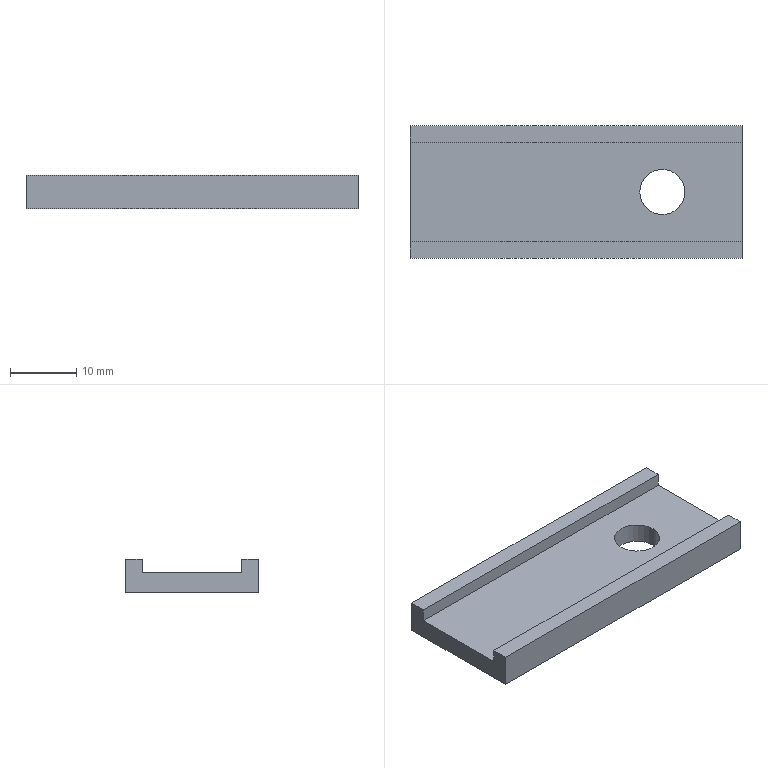Part | STEP file | Lead screw fixed block QY-1-17 | 1 solid | 12 faces | box 50 x 20 x 5 mm | volume 3391 mm3 | plane 10 | cylinder 2 | commonest cylinder face diameters 6.8 x2
STEP:
#1=CARTESIAN_POINT('',(0.,0.,0.));
#2=DIRECTION('',(0.,0.,1.));
#3=DIRECTION('',(1.,0.,0.));
#4=AXIS2_PLACEMENT_3D('',#1,#2,#3);
#5=CARTESIAN_POINT('',(16.4,0.,0.));
#6=VERTEX_POINT('',#5);
#7=CARTESIAN_POINT('',(16.4,0.,3.));
#8=VERTEX_POINT('',#7);
#9=CARTESIAN_POINT('',(16.4,0.,3.));
#10=DIRECTION('',(0.,0.,1.));
#11=VECTOR('',#10,1.);
#12=LINE('',#9,#11);
#13=CARTESIAN_POINT('',(13.,0.,3.));
#14=DIRECTION('',(0.,0.,1.));
#15=DIRECTION('',(1.,0.,0.));
#16=AXIS2_PLACEMENT_3D('',#13,#14,#15);
#17=CYLINDRICAL_SURFACE('',#16,3.4);
#18=CARTESIAN_POINT('',(6.283,0.));
#19=DIRECTION('',(0.,1.));
#20=VECTOR('',#19,1.);
#21=LINE('',#18,#20);
#22=(GEOMETRIC_REPRESENTATION_CONTEXT(2)PARAMETRIC_REPRESENTATION_CONTEXT()REPRESENTATION_CONTEXT('',''));
#23=DEFINITIONAL_REPRESENTATION('',(#21),#22);
#24=PCURVE('',#17,#23);
#25=CARTESIAN_POINT('',(13.,0.,3.));
#26=DIRECTION('',(0.,0.,1.));
#27=DIRECTION('',(1.,0.,0.));
#28=AXIS2_PLACEMENT_3D('',#25,#26,#27);
#29=CYLINDRICAL_SURFACE('',#28,3.4);
#30=CARTESIAN_POINT('',(0.,0.));
#31=DIRECTION('',(0.,1.));
#32=VECTOR('',#31,1.);
#33=LINE('',#30,#32);
#34=(GEOMETRIC_REPRESENTATION_CONTEXT(2)PARAMETRIC_REPRESENTATION_CONTEXT()REPRESENTATION_CONTEXT('',''));
#35=DEFINITIONAL_REPRESENTATION('',(#33),#34);
#36=PCURVE('',#29,#35);
#37=SURFACE_CURVE('',#12,(#24,#36),.PCURVE_S1.);
#38=EDGE_CURVE('',#6,#8,#37,.T.);
#39=ORIENTED_EDGE('',*,*,#38,.T.);
#40=CARTESIAN_POINT('',(9.6,0.,3.));
#41=VERTEX_POINT('',#40);
#42=CARTESIAN_POINT('',(13.,0.,3.));
#43=DIRECTION('',(0.,0.,1.));
#44=DIRECTION('',(1.,0.,0.));
#45=AXIS2_PLACEMENT_3D('',#42,#43,#44);
#46=CIRCLE('',#45,3.4);
#47=CARTESIAN_POINT('',(0.,0.));
#48=DIRECTION('',(1.,0.));
#49=VECTOR('',#48,1.);
#50=LINE('',#47,#49);
#51=(GEOMETRIC_REPRESENTATION_CONTEXT(2)PARAMETRIC_REPRESENTATION_CONTEXT()REPRESENTATION_CONTEXT('',''));
#52=DEFINITIONAL_REPRESENTATION('',(#50),#51);
#53=PCURVE('',#17,#52);
#54=CARTESIAN_POINT('',(0.,0.,3.));
#55=DIRECTION('',(0.,0.,-1.));
#56=DIRECTION('',(-1.,0.,0.));
#57=AXIS2_PLACEMENT_3D('',#54,#55,#56);
#58=PLANE('',#57);
#59=CARTESIAN_POINT('',(-16.4,0.));
#60=CARTESIAN_POINT('',(-16.4,5.889));
#61=CARTESIAN_POINT('',(-11.3,2.944));
#62=CARTESIAN_POINT('',(-6.2,0.));
#63=CARTESIAN_POINT('',(-11.3,-2.944));
#64=CARTESIAN_POINT('',(-16.4,-5.889));
#65=CARTESIAN_POINT('',(-16.4,0.));
#66=(BOUNDED_CURVE()B_SPLINE_CURVE(2,(#59,#60,#61,#62,#63,#64,#65),.UNSPECIFIED.,.T.,.F.)B_SPLINE_CURVE_WITH_KNOTS((1,2,2,2,2,1),(-2.094,0.,2.094,4.189,6.283,8.378),.UNSPECIFIED.)CURVE()GEOMETRIC_REPRESENTATION_ITEM()RATIONAL_B_SPLINE_CURVE((1.,0.5,1.,0.5,1.,0.5,1.))REPRESENTATION_ITEM(''));
#67=(GEOMETRIC_REPRESENTATION_CONTEXT(2)PARAMETRIC_REPRESENTATION_CONTEXT()REPRESENTATION_CONTEXT('',''));
#68=DEFINITIONAL_REPRESENTATION('',(#66),#67);
#69=PCURVE('',#58,#68);
#70=SURFACE_CURVE('',#46,(#53,#69),.PCURVE_S1.);
#71=EDGE_CURVE('',#41,#8,#70,.T.);
#72=ORIENTED_EDGE('',*,*,#71,.F.);
#73=CARTESIAN_POINT('',(9.6,0.,0.));
#74=VERTEX_POINT('',#73);
#75=CARTESIAN_POINT('',(9.6,0.,3.));
#76=DIRECTION('',(0.,0.,1.));
#77=VECTOR('',#76,1.);
#78=LINE('',#75,#77);
#79=CARTESIAN_POINT('',(3.142,0.));
#80=DIRECTION('',(0.,1.));
#81=VECTOR('',#80,1.);
#82=LINE('',#79,#81);
#83=(GEOMETRIC_REPRESENTATION_CONTEXT(2)PARAMETRIC_REPRESENTATION_CONTEXT()REPRESENTATION_CONTEXT('',''));
#84=DEFINITIONAL_REPRESENTATION('',(#82),#83);
#85=PCURVE('',#17,#84);
#86=CARTESIAN_POINT('',(3.142,0.));
#87=DIRECTION('',(0.,1.));
#88=VECTOR('',#87,1.);
#89=LINE('',#86,#88);
#90=(GEOMETRIC_REPRESENTATION_CONTEXT(2)PARAMETRIC_REPRESENTATION_CONTEXT()REPRESENTATION_CONTEXT('',''));
#91=DEFINITIONAL_REPRESENTATION('',(#89),#90);
#92=PCURVE('',#29,#91);
#93=SURFACE_CURVE('',#78,(#85,#92),.PCURVE_S1.);
#94=EDGE_CURVE('',#74,#41,#93,.T.);
#95=ORIENTED_EDGE('',*,*,#94,.F.);
#96=CARTESIAN_POINT('',(13.,0.,0.));
#97=DIRECTION('',(0.,0.,1.));
#98=DIRECTION('',(1.,0.,0.));
#99=AXIS2_PLACEMENT_3D('',#96,#97,#98);
#100=CIRCLE('',#99,3.4);
#101=CARTESIAN_POINT('',(0.,-3.));
#102=DIRECTION('',(1.,0.));
#103=VECTOR('',#102,1.);
#104=LINE('',#101,#103);
#105=(GEOMETRIC_REPRESENTATION_CONTEXT(2)PARAMETRIC_REPRESENTATION_CONTEXT()REPRESENTATION_CONTEXT('',''));
#106=DEFINITIONAL_REPRESENTATION('',(#104),#105);
#107=PCURVE('',#17,#106);
#108=CARTESIAN_POINT('',(0.,0.,0.));
#109=DIRECTION('',(0.,0.,1.));
#110=DIRECTION('',(1.,0.,0.));
#111=AXIS2_PLACEMENT_3D('',#108,#109,#110);
#112=PLANE('',#111);
#113=CARTESIAN_POINT('',(13.,0.));
#114=DIRECTION('',(1.,0.));
#115=AXIS2_PLACEMENT_2D('',#113,#114);
#116=CIRCLE('',#115,3.4);
#117=(GEOMETRIC_REPRESENTATION_CONTEXT(2)PARAMETRIC_REPRESENTATION_CONTEXT()REPRESENTATION_CONTEXT('',''));
#118=DEFINITIONAL_REPRESENTATION('',(#116),#117);
#119=PCURVE('',#112,#118);
#120=SURFACE_CURVE('',#100,(#107,#119),.PCURVE_S1.);
#121=EDGE_CURVE('',#74,#6,#120,.T.);
#122=ORIENTED_EDGE('',*,*,#121,.T.);
#123=EDGE_LOOP('',(#39,#72,#95,#122));
#124=FACE_BOUND('',#123,.F.);
#125=ADVANCED_FACE('',(#124),#17,.F.);
#126=CARTESIAN_POINT('',(-25.,-7.5,5.));
#127=VERTEX_POINT('',#126);
#128=CARTESIAN_POINT('',(25.,-7.5,5.));
#129=VERTEX_POINT('',#128);
#130=CARTESIAN_POINT('',(0.,-7.5,5.));
#131=DIRECTION('',(1.,0.,0.));
#132=VECTOR('',#131,1.);
#133=LINE('',#130,#132);
#134=CARTESIAN_POINT('',(0.,0.,5.));
#135=DIRECTION('',(0.,0.,1.));
#136=DIRECTION('',(1.,0.,0.));
#137=AXIS2_PLACEMENT_3D('',#134,#135,#136);
#138=PLANE('',#137);
#139=CARTESIAN_POINT('',(0.,-7.5));
#140=DIRECTION('',(1.,0.));
#141=VECTOR('',#140,1.);
#142=LINE('',#139,#141);
#143=(GEOMETRIC_REPRESENTATION_CONTEXT(2)PARAMETRIC_REPRESENTATION_CONTEXT()REPRESENTATION_CONTEXT('',''));
#144=DEFINITIONAL_REPRESENTATION('',(#142),#143);
#145=PCURVE('',#138,#144);
#146=CARTESIAN_POINT('',(-35.049,-7.5,3.));
#147=DIRECTION('',(0.,-1.,0.));
#148=DIRECTION('',(0.,0.,-1.));
#149=AXIS2_PLACEMENT_3D('',#146,#147,#148);
#150=PLANE('',#149);
#151=CARTESIAN_POINT('',(-2.,35.049));
#152=DIRECTION('',(0.,1.));
#153=VECTOR('',#152,1.);
#154=LINE('',#151,#153);
#155=(GEOMETRIC_REPRESENTATION_CONTEXT(2)PARAMETRIC_REPRESENTATION_CONTEXT()REPRESENTATION_CONTEXT('',''));
#156=DEFINITIONAL_REPRESENTATION('',(#154),#155);
#157=PCURVE('',#150,#156);
#158=SURFACE_CURVE('',#133,(#145,#157),.PCURVE_S1.);
#159=EDGE_CURVE('',#127,#129,#158,.T.);
#160=ORIENTED_EDGE('',*,*,#159,.F.);
#161=CARTESIAN_POINT('',(-25.,-10.,5.));
#162=VERTEX_POINT('',#161);
#163=CARTESIAN_POINT('',(-25.,10.,5.));
#164=DIRECTION('',(0.,-1.,0.));
#165=VECTOR('',#164,1.);
#166=LINE('',#163,#165);
#167=CARTESIAN_POINT('',(-25.,10.));
#168=DIRECTION('',(0.,-1.));
#169=VECTOR('',#168,1.);
#170=LINE('',#167,#169);
#171=(GEOMETRIC_REPRESENTATION_CONTEXT(2)PARAMETRIC_REPRESENTATION_CONTEXT()REPRESENTATION_CONTEXT('',''));
#172=DEFINITIONAL_REPRESENTATION('',(#170),#171);
#173=PCURVE('',#138,#172);
#174=CARTESIAN_POINT('',(-25.,10.,5.));
#175=DIRECTION('',(1.,0.,0.));
#176=DIRECTION('',(0.,0.,-1.));
#177=AXIS2_PLACEMENT_3D('',#174,#175,#176);
#178=PLANE('',#177);
#179=CARTESIAN_POINT('',(0.,0.));
#180=DIRECTION('',(0.,-1.));
#181=VECTOR('',#180,1.);
#182=LINE('',#179,#181);
#183=(GEOMETRIC_REPRESENTATION_CONTEXT(2)PARAMETRIC_REPRESENTATION_CONTEXT()REPRESENTATION_CONTEXT('',''));
#184=DEFINITIONAL_REPRESENTATION('',(#182),#183);
#185=PCURVE('',#178,#184);
#186=SURFACE_CURVE('',#166,(#173,#185),.PCURVE_S1.);
#187=EDGE_CURVE('',#127,#162,#186,.T.);
#188=ORIENTED_EDGE('',*,*,#187,.T.);
#189=CARTESIAN_POINT('',(25.,-10.,5.));
#190=VERTEX_POINT('',#189);
#191=CARTESIAN_POINT('',(-25.,-10.,5.));
#192=DIRECTION('',(1.,0.,0.));
#193=VECTOR('',#192,1.);
#194=LINE('',#191,#193);
#195=CARTESIAN_POINT('',(-25.,-10.));
#196=DIRECTION('',(1.,0.));
#197=VECTOR('',#196,1.);
#198=LINE('',#195,#197);
#199=(GEOMETRIC_REPRESENTATION_CONTEXT(2)PARAMETRIC_REPRESENTATION_CONTEXT()REPRESENTATION_CONTEXT('',''));
#200=DEFINITIONAL_REPRESENTATION('',(#198),#199);
#201=PCURVE('',#138,#200);
#202=CARTESIAN_POINT('',(-25.,-10.,5.));
#203=DIRECTION('',(0.,1.,0.));
#204=DIRECTION('',(0.,0.,1.));
#205=AXIS2_PLACEMENT_3D('',#202,#203,#204);
#206=PLANE('',#205);
#207=CARTESIAN_POINT('',(0.,0.));
#208=DIRECTION('',(0.,1.));
#209=VECTOR('',#208,1.);
#210=LINE('',#207,#209);
#211=(GEOMETRIC_REPRESENTATION_CONTEXT(2)PARAMETRIC_REPRESENTATION_CONTEXT()REPRESENTATION_CONTEXT('',''));
#212=DEFINITIONAL_REPRESENTATION('',(#210),#211);
#213=PCURVE('',#206,#212);
#214=SURFACE_CURVE('',#194,(#201,#213),.PCURVE_S1.);
#215=EDGE_CURVE('',#162,#190,#214,.T.);
#216=ORIENTED_EDGE('',*,*,#215,.T.);
#217=CARTESIAN_POINT('',(25.,10.,5.));
#218=DIRECTION('',(0.,1.,0.));
#219=VECTOR('',#218,1.);
#220=LINE('',#217,#219);
#221=CARTESIAN_POINT('',(25.,10.));
#222=DIRECTION('',(0.,1.));
#223=VECTOR('',#222,1.);
#224=LINE('',#221,#223);
#225=(GEOMETRIC_REPRESENTATION_CONTEXT(2)PARAMETRIC_REPRESENTATION_CONTEXT()REPRESENTATION_CONTEXT('',''));
#226=DEFINITIONAL_REPRESENTATION('',(#224),#225);
#227=PCURVE('',#138,#226);
#228=CARTESIAN_POINT('',(25.,10.,5.));
#229=DIRECTION('',(-1.,0.,0.));
#230=DIRECTION('',(0.,-1.,0.));
#231=AXIS2_PLACEMENT_3D('',#228,#229,#230);
#232=PLANE('',#231);
#233=CARTESIAN_POINT('',(0.,0.));
#234=DIRECTION('',(-1.,0.));
#235=VECTOR('',#234,1.);
#236=LINE('',#233,#235);
#237=(GEOMETRIC_REPRESENTATION_CONTEXT(2)PARAMETRIC_REPRESENTATION_CONTEXT()REPRESENTATION_CONTEXT('',''));
#238=DEFINITIONAL_REPRESENTATION('',(#236),#237);
#239=PCURVE('',#232,#238);
#240=SURFACE_CURVE('',#220,(#227,#239),.PCURVE_S1.);
#241=EDGE_CURVE('',#190,#129,#240,.T.);
#242=ORIENTED_EDGE('',*,*,#241,.T.);
#243=EDGE_LOOP('',(#160,#188,#216,#242));
#244=FACE_BOUND('',#243,.T.);
#245=ADVANCED_FACE('',(#244),#138,.T.);
#246=CARTESIAN_POINT('',(25.,7.5,3.));
#247=VERTEX_POINT('',#246);
#248=CARTESIAN_POINT('',(25.,-7.5,3.));
#249=VERTEX_POINT('',#248);
#250=CARTESIAN_POINT('',(25.,10.,3.));
#251=DIRECTION('',(0.,-1.,0.));
#252=VECTOR('',#251,1.);
#253=LINE('',#250,#252);
#254=CARTESIAN_POINT('',(0.,-2.));
#255=DIRECTION('',(1.,0.));
#256=VECTOR('',#255,1.);
#257=LINE('',#254,#256);
#258=(GEOMETRIC_REPRESENTATION_CONTEXT(2)PARAMETRIC_REPRESENTATION_CONTEXT()REPRESENTATION_CONTEXT('',''));
#259=DEFINITIONAL_REPRESENTATION('',(#257),#258);
#260=PCURVE('',#232,#259);
#261=CARTESIAN_POINT('',(-25.,10.));
#262=DIRECTION('',(0.,-1.));
#263=VECTOR('',#262,1.);
#264=LINE('',#261,#263);
#265=(GEOMETRIC_REPRESENTATION_CONTEXT(2)PARAMETRIC_REPRESENTATION_CONTEXT()REPRESENTATION_CONTEXT('',''));
#266=DEFINITIONAL_REPRESENTATION('',(#264),#265);
#267=PCURVE('',#58,#266);
#268=SURFACE_CURVE('',#253,(#260,#267),.PCURVE_S1.);
#269=EDGE_CURVE('',#247,#249,#268,.T.);
#270=ORIENTED_EDGE('',*,*,#269,.T.);
#271=CARTESIAN_POINT('',(25.,-7.5,5.));
#272=DIRECTION('',(0.,0.,1.));
#273=VECTOR('',#272,1.);
#274=LINE('',#271,#273);
#275=CARTESIAN_POINT('',(17.5,0.));
#276=DIRECTION('',(0.,1.));
#277=VECTOR('',#276,1.);
#278=LINE('',#275,#277);
#279=(GEOMETRIC_REPRESENTATION_CONTEXT(2)PARAMETRIC_REPRESENTATION_CONTEXT()REPRESENTATION_CONTEXT('',''));
#280=DEFINITIONAL_REPRESENTATION('',(#278),#279);
#281=PCURVE('',#232,#280);
#282=CARTESIAN_POINT('',(-2.,60.049));
#283=DIRECTION('',(-1.,0.));
#284=VECTOR('',#283,1.);
#285=LINE('',#282,#284);
#286=(GEOMETRIC_REPRESENTATION_CONTEXT(2)PARAMETRIC_REPRESENTATION_CONTEXT()REPRESENTATION_CONTEXT('',''));
#287=DEFINITIONAL_REPRESENTATION('',(#285),#286);
#288=PCURVE('',#150,#287);
#289=SURFACE_CURVE('',#274,(#281,#288),.PCURVE_S1.);
#290=EDGE_CURVE('',#249,#129,#289,.T.);
#291=ORIENTED_EDGE('',*,*,#290,.T.);
#292=ORIENTED_EDGE('',*,*,#241,.F.);
#293=CARTESIAN_POINT('',(25.,-10.,0.));
#294=VERTEX_POINT('',#293);
#295=CARTESIAN_POINT('',(25.,-10.,5.));
#296=DIRECTION('',(0.,0.,-1.));
#297=VECTOR('',#296,1.);
#298=LINE('',#295,#297);
#299=CARTESIAN_POINT('',(20.,0.));
#300=DIRECTION('',(0.,-1.));
#301=VECTOR('',#300,1.);
#302=LINE('',#299,#301);
#303=(GEOMETRIC_REPRESENTATION_CONTEXT(2)PARAMETRIC_REPRESENTATION_CONTEXT()REPRESENTATION_CONTEXT('',''));
#304=DEFINITIONAL_REPRESENTATION('',(#302),#303);
#305=PCURVE('',#232,#304);
#306=CARTESIAN_POINT('',(0.,50.));
#307=DIRECTION('',(-1.,0.));
#308=VECTOR('',#307,1.);
#309=LINE('',#306,#308);
#310=(GEOMETRIC_REPRESENTATION_CONTEXT(2)PARAMETRIC_REPRESENTATION_CONTEXT()REPRESENTATION_CONTEXT('',''));
#311=DEFINITIONAL_REPRESENTATION('',(#309),#310);
#312=PCURVE('',#206,#311);
#313=SURFACE_CURVE('',#298,(#305,#312),.PCURVE_S1.);
#314=EDGE_CURVE('',#190,#294,#313,.T.);
#315=ORIENTED_EDGE('',*,*,#314,.T.);
#316=CARTESIAN_POINT('',(25.,10.,0.));
#317=VERTEX_POINT('',#316);
#318=CARTESIAN_POINT('',(25.,10.,0.));
#319=DIRECTION('',(0.,1.,0.));
#320=VECTOR('',#319,1.);
#321=LINE('',#318,#320);
#322=CARTESIAN_POINT('',(0.,-5.));
#323=DIRECTION('',(-1.,0.));
#324=VECTOR('',#323,1.);
#325=LINE('',#322,#324);
#326=(GEOMETRIC_REPRESENTATION_CONTEXT(2)PARAMETRIC_REPRESENTATION_CONTEXT()REPRESENTATION_CONTEXT('',''));
#327=DEFINITIONAL_REPRESENTATION('',(#325),#326);
#328=PCURVE('',#232,#327);
#329=CARTESIAN_POINT('',(25.,10.));
#330=DIRECTION('',(0.,1.));
#331=VECTOR('',#330,1.);
#332=LINE('',#329,#331);
#333=(GEOMETRIC_REPRESENTATION_CONTEXT(2)PARAMETRIC_REPRESENTATION_CONTEXT()REPRESENTATION_CONTEXT('',''));
#334=DEFINITIONAL_REPRESENTATION('',(#332),#333);
#335=PCURVE('',#112,#334);
#336=SURFACE_CURVE('',#321,(#328,#335),.PCURVE_S1.);
#337=EDGE_CURVE('',#294,#317,#336,.T.);
#338=ORIENTED_EDGE('',*,*,#337,.T.);
#339=CARTESIAN_POINT('',(25.,10.,5.));
#340=VERTEX_POINT('',#339);
#341=CARTESIAN_POINT('',(25.,10.,5.));
#342=DIRECTION('',(0.,0.,-1.));
#343=VECTOR('',#342,1.);
#344=LINE('',#341,#343);
#345=CARTESIAN_POINT('',(0.,0.));
#346=DIRECTION('',(0.,-1.));
#347=VECTOR('',#346,1.);
#348=LINE('',#345,#347);
#349=(GEOMETRIC_REPRESENTATION_CONTEXT(2)PARAMETRIC_REPRESENTATION_CONTEXT()REPRESENTATION_CONTEXT('',''));
#350=DEFINITIONAL_REPRESENTATION('',(#348),#349);
#351=PCURVE('',#232,#350);
#352=CARTESIAN_POINT('',(-25.,10.,5.));
#353=DIRECTION('',(0.,-1.,0.));
#354=DIRECTION('',(0.,0.,-1.));
#355=AXIS2_PLACEMENT_3D('',#352,#353,#354);
#356=PLANE('',#355);
#357=CARTESIAN_POINT('',(0.,50.));
#358=DIRECTION('',(1.,0.));
#359=VECTOR('',#358,1.);
#360=LINE('',#357,#359);
#361=(GEOMETRIC_REPRESENTATION_CONTEXT(2)PARAMETRIC_REPRESENTATION_CONTEXT()REPRESENTATION_CONTEXT('',''));
#362=DEFINITIONAL_REPRESENTATION('',(#360),#361);
#363=PCURVE('',#356,#362);
#364=SURFACE_CURVE('',#344,(#351,#363),.PCURVE_S1.);
#365=EDGE_CURVE('',#340,#317,#364,.T.);
#366=ORIENTED_EDGE('',*,*,#365,.F.);
#367=CARTESIAN_POINT('',(25.,7.5,5.));
#368=VERTEX_POINT('',#367);
#369=CARTESIAN_POINT('',(25.,10.,5.));
#370=DIRECTION('',(0.,1.,0.));
#371=VECTOR('',#370,1.);
#372=LINE('',#369,#371);
#373=CARTESIAN_POINT('',(0.,0.));
#374=DIRECTION('',(-1.,0.));
#375=VECTOR('',#374,1.);
#376=LINE('',#373,#375);
#377=(GEOMETRIC_REPRESENTATION_CONTEXT(2)PARAMETRIC_REPRESENTATION_CONTEXT()REPRESENTATION_CONTEXT('',''));
#378=DEFINITIONAL_REPRESENTATION('',(#376),#377);
#379=PCURVE('',#232,#378);
#380=CARTESIAN_POINT('',(0.,0.,5.));
#381=DIRECTION('',(0.,0.,1.));
#382=DIRECTION('',(1.,0.,0.));
#383=AXIS2_PLACEMENT_3D('',#380,#381,#382);
#384=PLANE('',#383);
#385=CARTESIAN_POINT('',(25.,10.));
#386=DIRECTION('',(0.,1.));
#387=VECTOR('',#386,1.);
#388=LINE('',#385,#387);
#389=(GEOMETRIC_REPRESENTATION_CONTEXT(2)PARAMETRIC_REPRESENTATION_CONTEXT()REPRESENTATION_CONTEXT('',''));
#390=DEFINITIONAL_REPRESENTATION('',(#388),#389);
#391=PCURVE('',#384,#390);
#392=SURFACE_CURVE('',#372,(#379,#391),.PCURVE_S1.);
#393=EDGE_CURVE('',#368,#340,#392,.T.);
#394=ORIENTED_EDGE('',*,*,#393,.F.);
#395=CARTESIAN_POINT('',(25.,7.5,5.));
#396=DIRECTION('',(0.,0.,-1.));
#397=VECTOR('',#396,1.);
#398=LINE('',#395,#397);
#399=CARTESIAN_POINT('',(2.5,0.));
#400=DIRECTION('',(0.,-1.));
#401=VECTOR('',#400,1.);
#402=LINE('',#399,#401);
#403=(GEOMETRIC_REPRESENTATION_CONTEXT(2)PARAMETRIC_REPRESENTATION_CONTEXT()REPRESENTATION_CONTEXT('',''));
#404=DEFINITIONAL_REPRESENTATION('',(#402),#403);
#405=PCURVE('',#232,#404);
#406=CARTESIAN_POINT('',(-35.049,7.5,3.));
#407=DIRECTION('',(0.,1.,0.));
#408=DIRECTION('',(0.,0.,1.));
#409=AXIS2_PLACEMENT_3D('',#406,#407,#408);
#410=PLANE('',#409);
#411=CARTESIAN_POINT('',(2.,60.049));
#412=DIRECTION('',(-1.,0.));
#413=VECTOR('',#412,1.);
#414=LINE('',#411,#413);
#415=(GEOMETRIC_REPRESENTATION_CONTEXT(2)PARAMETRIC_REPRESENTATION_CONTEXT()REPRESENTATION_CONTEXT('',''));
#416=DEFINITIONAL_REPRESENTATION('',(#414),#415);
#417=PCURVE('',#410,#416);
#418=SURFACE_CURVE('',#398,(#405,#417),.PCURVE_S1.);
#419=EDGE_CURVE('',#368,#247,#418,.T.);
#420=ORIENTED_EDGE('',*,*,#419,.T.);
#421=EDGE_LOOP('',(#270,#291,#292,#315,#338,#366,#394,#420));
#422=FACE_BOUND('',#421,.T.);
#423=ADVANCED_FACE('',(#422),#232,.F.);
#424=CARTESIAN_POINT('',(-25.,10.,0.));
#425=VERTEX_POINT('',#424);
#426=CARTESIAN_POINT('',(-25.,10.,0.));
#427=DIRECTION('',(-1.,0.,0.));
#428=VECTOR('',#427,1.);
#429=LINE('',#426,#428);
#430=CARTESIAN_POINT('',(5.,0.));
#431=DIRECTION('',(0.,-1.));
#432=VECTOR('',#431,1.);
#433=LINE('',#430,#432);
#434=(GEOMETRIC_REPRESENTATION_CONTEXT(2)PARAMETRIC_REPRESENTATION_CONTEXT()REPRESENTATION_CONTEXT('',''));
#435=DEFINITIONAL_REPRESENTATION('',(#433),#434);
#436=PCURVE('',#356,#435);
#437=CARTESIAN_POINT('',(-25.,10.));
#438=DIRECTION('',(-1.,0.));
#439=VECTOR('',#438,1.);
#440=LINE('',#437,#439);
#441=(GEOMETRIC_REPRESENTATION_CONTEXT(2)PARAMETRIC_REPRESENTATION_CONTEXT()REPRESENTATION_CONTEXT('',''));
#442=DEFINITIONAL_REPRESENTATION('',(#440),#441);
#443=PCURVE('',#112,#442);
#444=SURFACE_CURVE('',#429,(#436,#443),.PCURVE_S1.);
#445=EDGE_CURVE('',#317,#425,#444,.T.);
#446=ORIENTED_EDGE('',*,*,#445,.T.);
#447=CARTESIAN_POINT('',(-25.,10.,5.));
#448=VERTEX_POINT('',#447);
#449=CARTESIAN_POINT('',(-25.,10.,5.));
#450=DIRECTION('',(0.,0.,-1.));
#451=VECTOR('',#450,1.);
#452=LINE('',#449,#451);
#453=CARTESIAN_POINT('',(0.,0.));
#454=DIRECTION('',(1.,0.));
#455=VECTOR('',#454,1.);
#456=LINE('',#453,#455);
#457=(GEOMETRIC_REPRESENTATION_CONTEXT(2)PARAMETRIC_REPRESENTATION_CONTEXT()REPRESENTATION_CONTEXT('',''));
#458=DEFINITIONAL_REPRESENTATION('',(#456),#457);
#459=PCURVE('',#356,#458);
#460=CARTESIAN_POINT('',(0.,0.));
#461=DIRECTION('',(1.,0.));
#462=VECTOR('',#461,1.);
#463=LINE('',#460,#462);
#464=(GEOMETRIC_REPRESENTATION_CONTEXT(2)PARAMETRIC_REPRESENTATION_CONTEXT()REPRESENTATION_CONTEXT('',''));
#465=DEFINITIONAL_REPRESENTATION('',(#463),#464);
#466=PCURVE('',#178,#465);
#467=SURFACE_CURVE('',#452,(#459,#466),.PCURVE_S1.);
#468=EDGE_CURVE('',#448,#425,#467,.T.);
#469=ORIENTED_EDGE('',*,*,#468,.F.);
#470=CARTESIAN_POINT('',(-25.,10.,5.));
#471=DIRECTION('',(-1.,0.,0.));
#472=VECTOR('',#471,1.);
#473=LINE('',#470,#472);
#474=CARTESIAN_POINT('',(0.,0.));
#475=DIRECTION('',(0.,-1.));
#476=VECTOR('',#475,1.);
#477=LINE('',#474,#476);
#478=(GEOMETRIC_REPRESENTATION_CONTEXT(2)PARAMETRIC_REPRESENTATION_CONTEXT()REPRESENTATION_CONTEXT('',''));
#479=DEFINITIONAL_REPRESENTATION('',(#477),#478);
#480=PCURVE('',#356,#479);
#481=CARTESIAN_POINT('',(-25.,10.));
#482=DIRECTION('',(-1.,0.));
#483=VECTOR('',#482,1.);
#484=LINE('',#481,#483);
#485=(GEOMETRIC_REPRESENTATION_CONTEXT(2)PARAMETRIC_REPRESENTATION_CONTEXT()REPRESENTATION_CONTEXT('',''));
#486=DEFINITIONAL_REPRESENTATION('',(#484),#485);
#487=PCURVE('',#384,#486);
#488=SURFACE_CURVE('',#473,(#480,#487),.PCURVE_S1.);
#489=EDGE_CURVE('',#340,#448,#488,.T.);
#490=ORIENTED_EDGE('',*,*,#489,.F.);
#491=ORIENTED_EDGE('',*,*,#365,.T.);
#492=EDGE_LOOP('',(#446,#469,#490,#491));
#493=FACE_BOUND('',#492,.T.);
#494=ADVANCED_FACE('',(#493),#356,.F.);
#495=ORIENTED_EDGE('',*,*,#187,.F.);
#496=CARTESIAN_POINT('',(-25.,-7.5,3.));
#497=VERTEX_POINT('',#496);
#498=CARTESIAN_POINT('',(-25.,-7.5,5.));
#499=DIRECTION('',(0.,0.,-1.));
#500=VECTOR('',#499,1.);
#501=LINE('',#498,#500);
#502=CARTESIAN_POINT('',(0.,-17.5));
#503=DIRECTION('',(1.,0.));
#504=VECTOR('',#503,1.);
#505=LINE('',#502,#504);
#506=(GEOMETRIC_REPRESENTATION_CONTEXT(2)PARAMETRIC_REPRESENTATION_CONTEXT()REPRESENTATION_CONTEXT('',''));
#507=DEFINITIONAL_REPRESENTATION('',(#505),#506);
#508=PCURVE('',#178,#507);
#509=CARTESIAN_POINT('',(-2.,10.049));
#510=DIRECTION('',(1.,0.));
#511=VECTOR('',#510,1.);
#512=LINE('',#509,#511);
#513=(GEOMETRIC_REPRESENTATION_CONTEXT(2)PARAMETRIC_REPRESENTATION_CONTEXT()REPRESENTATION_CONTEXT('',''));
#514=DEFINITIONAL_REPRESENTATION('',(#512),#513);
#515=PCURVE('',#150,#514);
#516=SURFACE_CURVE('',#501,(#508,#515),.PCURVE_S1.);
#517=EDGE_CURVE('',#127,#497,#516,.T.);
#518=ORIENTED_EDGE('',*,*,#517,.T.);
#519=CARTESIAN_POINT('',(-25.,7.5,3.));
#520=VERTEX_POINT('',#519);
#521=CARTESIAN_POINT('',(-25.,10.,3.));
#522=DIRECTION('',(0.,1.,0.));
#523=VECTOR('',#522,1.);
#524=LINE('',#521,#523);
#525=CARTESIAN_POINT('',(2.,0.));
#526=DIRECTION('',(0.,1.));
#527=VECTOR('',#526,1.);
#528=LINE('',#525,#527);
#529=(GEOMETRIC_REPRESENTATION_CONTEXT(2)PARAMETRIC_REPRESENTATION_CONTEXT()REPRESENTATION_CONTEXT('',''));
#530=DEFINITIONAL_REPRESENTATION('',(#528),#529);
#531=PCURVE('',#178,#530);
#532=CARTESIAN_POINT('',(25.,10.));
#533=DIRECTION('',(0.,1.));
#534=VECTOR('',#533,1.);
#535=LINE('',#532,#534);
#536=(GEOMETRIC_REPRESENTATION_CONTEXT(2)PARAMETRIC_REPRESENTATION_CONTEXT()REPRESENTATION_CONTEXT('',''));
#537=DEFINITIONAL_REPRESENTATION('',(#535),#536);
#538=PCURVE('',#58,#537);
#539=SURFACE_CURVE('',#524,(#531,#538),.PCURVE_S1.);
#540=EDGE_CURVE('',#497,#520,#539,.T.);
#541=ORIENTED_EDGE('',*,*,#540,.T.);
#542=CARTESIAN_POINT('',(-25.,7.5,5.));
#543=VERTEX_POINT('',#542);
#544=CARTESIAN_POINT('',(-25.,7.5,5.));
#545=DIRECTION('',(0.,0.,1.));
#546=VECTOR('',#545,1.);
#547=LINE('',#544,#546);
#548=CARTESIAN_POINT('',(0.,-2.5));
#549=DIRECTION('',(-1.,0.));
#550=VECTOR('',#549,1.);
#551=LINE('',#548,#550);
#552=(GEOMETRIC_REPRESENTATION_CONTEXT(2)PARAMETRIC_REPRESENTATION_CONTEXT()REPRESENTATION_CONTEXT('',''));
#553=DEFINITIONAL_REPRESENTATION('',(#551),#552);
#554=PCURVE('',#178,#553);
#555=CARTESIAN_POINT('',(2.,10.049));
#556=DIRECTION('',(1.,0.));
#557=VECTOR('',#556,1.);
#558=LINE('',#555,#557);
#559=(GEOMETRIC_REPRESENTATION_CONTEXT(2)PARAMETRIC_REPRESENTATION_CONTEXT()REPRESENTATION_CONTEXT('',''));
#560=DEFINITIONAL_REPRESENTATION('',(#558),#559);
#561=PCURVE('',#410,#560);
#562=SURFACE_CURVE('',#547,(#554,#561),.PCURVE_S1.);
#563=EDGE_CURVE('',#520,#543,#562,.T.);
#564=ORIENTED_EDGE('',*,*,#563,.T.);
#565=CARTESIAN_POINT('',(-25.,10.,5.));
#566=DIRECTION('',(0.,-1.,0.));
#567=VECTOR('',#566,1.);
#568=LINE('',#565,#567);
#569=CARTESIAN_POINT('',(0.,0.));
#570=DIRECTION('',(0.,-1.));
#571=VECTOR('',#570,1.);
#572=LINE('',#569,#571);
#573=(GEOMETRIC_REPRESENTATION_CONTEXT(2)PARAMETRIC_REPRESENTATION_CONTEXT()REPRESENTATION_CONTEXT('',''));
#574=DEFINITIONAL_REPRESENTATION('',(#572),#573);
#575=PCURVE('',#178,#574);
#576=CARTESIAN_POINT('',(-25.,10.));
#577=DIRECTION('',(0.,-1.));
#578=VECTOR('',#577,1.);
#579=LINE('',#576,#578);
#580=(GEOMETRIC_REPRESENTATION_CONTEXT(2)PARAMETRIC_REPRESENTATION_CONTEXT()REPRESENTATION_CONTEXT('',''));
#581=DEFINITIONAL_REPRESENTATION('',(#579),#580);
#582=PCURVE('',#384,#581);
#583=SURFACE_CURVE('',#568,(#575,#582),.PCURVE_S1.);
#584=EDGE_CURVE('',#448,#543,#583,.T.);
#585=ORIENTED_EDGE('',*,*,#584,.F.);
#586=ORIENTED_EDGE('',*,*,#468,.T.);
#587=CARTESIAN_POINT('',(-25.,-10.,0.));
#588=VERTEX_POINT('',#587);
#589=CARTESIAN_POINT('',(-25.,10.,0.));
#590=DIRECTION('',(0.,-1.,0.));
#591=VECTOR('',#590,1.);
#592=LINE('',#589,#591);
#593=CARTESIAN_POINT('',(5.,0.));
#594=DIRECTION('',(0.,-1.));
#595=VECTOR('',#594,1.);
#596=LINE('',#593,#595);
#597=(GEOMETRIC_REPRESENTATION_CONTEXT(2)PARAMETRIC_REPRESENTATION_CONTEXT()REPRESENTATION_CONTEXT('',''));
#598=DEFINITIONAL_REPRESENTATION('',(#596),#597);
#599=PCURVE('',#178,#598);
#600=CARTESIAN_POINT('',(-25.,10.));
#601=DIRECTION('',(0.,-1.));
#602=VECTOR('',#601,1.);
#603=LINE('',#600,#602);
#604=(GEOMETRIC_REPRESENTATION_CONTEXT(2)PARAMETRIC_REPRESENTATION_CONTEXT()REPRESENTATION_CONTEXT('',''));
#605=DEFINITIONAL_REPRESENTATION('',(#603),#604);
#606=PCURVE('',#112,#605);
#607=SURFACE_CURVE('',#592,(#599,#606),.PCURVE_S1.);
#608=EDGE_CURVE('',#425,#588,#607,.T.);
#609=ORIENTED_EDGE('',*,*,#608,.T.);
#610=CARTESIAN_POINT('',(-25.,-10.,5.));
#611=DIRECTION('',(0.,0.,-1.));
#612=VECTOR('',#611,1.);
#613=LINE('',#610,#612);
#614=CARTESIAN_POINT('',(0.,-20.));
#615=DIRECTION('',(1.,0.));
#616=VECTOR('',#615,1.);
#617=LINE('',#614,#616);
#618=(GEOMETRIC_REPRESENTATION_CONTEXT(2)PARAMETRIC_REPRESENTATION_CONTEXT()REPRESENTATION_CONTEXT('',''));
#619=DEFINITIONAL_REPRESENTATION('',(#617),#618);
#620=PCURVE('',#178,#619);
#621=CARTESIAN_POINT('',(0.,0.));
#622=DIRECTION('',(-1.,0.));
#623=VECTOR('',#622,1.);
#624=LINE('',#621,#623);
#625=(GEOMETRIC_REPRESENTATION_CONTEXT(2)PARAMETRIC_REPRESENTATION_CONTEXT()REPRESENTATION_CONTEXT('',''));
#626=DEFINITIONAL_REPRESENTATION('',(#624),#625);
#627=PCURVE('',#206,#626);
#628=SURFACE_CURVE('',#613,(#620,#627),.PCURVE_S1.);
#629=EDGE_CURVE('',#162,#588,#628,.T.);
#630=ORIENTED_EDGE('',*,*,#629,.F.);
#631=EDGE_LOOP('',(#495,#518,#541,#564,#585,#586,#609,#630));
#632=FACE_BOUND('',#631,.T.);
#633=ADVANCED_FACE('',(#632),#178,.F.);
#634=CARTESIAN_POINT('',(-25.,-10.,0.));
#635=DIRECTION('',(1.,0.,0.));
#636=VECTOR('',#635,1.);
#637=LINE('',#634,#636);
#638=CARTESIAN_POINT('',(-5.,0.));
#639=DIRECTION('',(0.,1.));
#640=VECTOR('',#639,1.);
#641=LINE('',#638,#640);
#642=(GEOMETRIC_REPRESENTATION_CONTEXT(2)PARAMETRIC_REPRESENTATION_CONTEXT()REPRESENTATION_CONTEXT('',''));
#643=DEFINITIONAL_REPRESENTATION('',(#641),#642);
#644=PCURVE('',#206,#643);
#645=CARTESIAN_POINT('',(-25.,-10.));
#646=DIRECTION('',(1.,0.));
#647=VECTOR('',#646,1.);
#648=LINE('',#645,#647);
#649=(GEOMETRIC_REPRESENTATION_CONTEXT(2)PARAMETRIC_REPRESENTATION_CONTEXT()REPRESENTATION_CONTEXT('',''));
#650=DEFINITIONAL_REPRESENTATION('',(#648),#649);
#651=PCURVE('',#112,#650);
#652=SURFACE_CURVE('',#637,(#644,#651),.PCURVE_S1.);
#653=EDGE_CURVE('',#588,#294,#652,.T.);
#654=ORIENTED_EDGE('',*,*,#653,.T.);
#655=ORIENTED_EDGE('',*,*,#314,.F.);
#656=ORIENTED_EDGE('',*,*,#215,.F.);
#657=ORIENTED_EDGE('',*,*,#629,.T.);
#658=EDGE_LOOP('',(#654,#655,#656,#657));
#659=FACE_BOUND('',#658,.T.);
#660=ADVANCED_FACE('',(#659),#206,.F.);
#661=CARTESIAN_POINT('',(0.,7.5,5.));
#662=DIRECTION('',(-1.,0.,0.));
#663=VECTOR('',#662,1.);
#664=LINE('',#661,#663);
#665=CARTESIAN_POINT('',(0.,7.5));
#666=DIRECTION('',(-1.,0.));
#667=VECTOR('',#666,1.);
#668=LINE('',#665,#667);
#669=(GEOMETRIC_REPRESENTATION_CONTEXT(2)PARAMETRIC_REPRESENTATION_CONTEXT()REPRESENTATION_CONTEXT('',''));
#670=DEFINITIONAL_REPRESENTATION('',(#668),#669);
#671=PCURVE('',#384,#670);
#672=CARTESIAN_POINT('',(2.,35.049));
#673=DIRECTION('',(0.,-1.));
#674=VECTOR('',#673,1.);
#675=LINE('',#672,#674);
#676=(GEOMETRIC_REPRESENTATION_CONTEXT(2)PARAMETRIC_REPRESENTATION_CONTEXT()REPRESENTATION_CONTEXT('',''));
#677=DEFINITIONAL_REPRESENTATION('',(#675),#676);
#678=PCURVE('',#410,#677);
#679=SURFACE_CURVE('',#664,(#671,#678),.PCURVE_S1.);
#680=EDGE_CURVE('',#368,#543,#679,.T.);
#681=ORIENTED_EDGE('',*,*,#680,.F.);
#682=ORIENTED_EDGE('',*,*,#393,.T.);
#683=ORIENTED_EDGE('',*,*,#489,.T.);
#684=ORIENTED_EDGE('',*,*,#584,.T.);
#685=EDGE_LOOP('',(#681,#682,#683,#684));
#686=FACE_BOUND('',#685,.T.);
#687=ADVANCED_FACE('',(#686),#384,.T.);
#688=CARTESIAN_POINT('',(13.,0.,0.));
#689=DIRECTION('',(0.,0.,1.));
#690=DIRECTION('',(1.,0.,0.));
#691=AXIS2_PLACEMENT_3D('',#688,#689,#690);
#692=CIRCLE('',#691,3.4);
#693=CARTESIAN_POINT('',(13.,0.));
#694=DIRECTION('',(1.,0.));
#695=AXIS2_PLACEMENT_2D('',#693,#694);
#696=CIRCLE('',#695,3.4);
#697=(GEOMETRIC_REPRESENTATION_CONTEXT(2)PARAMETRIC_REPRESENTATION_CONTEXT()REPRESENTATION_CONTEXT('',''));
#698=DEFINITIONAL_REPRESENTATION('',(#696),#697);
#699=PCURVE('',#112,#698);
#700=CARTESIAN_POINT('',(0.,-3.));
#701=DIRECTION('',(1.,0.));
#702=VECTOR('',#701,1.);
#703=LINE('',#700,#702);
#704=(GEOMETRIC_REPRESENTATION_CONTEXT(2)PARAMETRIC_REPRESENTATION_CONTEXT()REPRESENTATION_CONTEXT('',''));
#705=DEFINITIONAL_REPRESENTATION('',(#703),#704);
#706=PCURVE('',#29,#705);
#707=SURFACE_CURVE('',#692,(#699,#706),.PCURVE_S1.);
#708=EDGE_CURVE('',#6,#74,#707,.T.);
#709=ORIENTED_EDGE('',*,*,#708,.T.);
#710=ORIENTED_EDGE('',*,*,#121,.T.);
#711=EDGE_LOOP('',(#709,#710));
#712=FACE_BOUND('',#711,.T.);
#713=ORIENTED_EDGE('',*,*,#337,.F.);
#714=ORIENTED_EDGE('',*,*,#653,.F.);
#715=ORIENTED_EDGE('',*,*,#608,.F.);
#716=ORIENTED_EDGE('',*,*,#445,.F.);
#717=EDGE_LOOP('',(#713,#714,#715,#716));
#718=FACE_BOUND('',#717,.T.);
#719=ADVANCED_FACE('',(#712,#718),#112,.F.);
#720=CARTESIAN_POINT('',(13.,0.,3.));
#721=DIRECTION('',(0.,0.,1.));
#722=DIRECTION('',(1.,0.,0.));
#723=AXIS2_PLACEMENT_3D('',#720,#721,#722);
#724=CIRCLE('',#723,3.4);
#725=CARTESIAN_POINT('',(-16.4,0.));
#726=CARTESIAN_POINT('',(-16.4,5.889));
#727=CARTESIAN_POINT('',(-11.3,2.944));
#728=CARTESIAN_POINT('',(-6.2,0.));
#729=CARTESIAN_POINT('',(-11.3,-2.944));
#730=CARTESIAN_POINT('',(-16.4,-5.889));
#731=CARTESIAN_POINT('',(-16.4,0.));
#732=(BOUNDED_CURVE()B_SPLINE_CURVE(2,(#725,#726,#727,#728,#729,#730,#731),.UNSPECIFIED.,.T.,.F.)B_SPLINE_CURVE_WITH_KNOTS((1,2,2,2,2,1),(-2.094,0.,2.094,4.189,6.283,8.378),.UNSPECIFIED.)CURVE()GEOMETRIC_REPRESENTATION_ITEM()RATIONAL_B_SPLINE_CURVE((1.,0.5,1.,0.5,1.,0.5,1.))REPRESENTATION_ITEM(''));
#733=(GEOMETRIC_REPRESENTATION_CONTEXT(2)PARAMETRIC_REPRESENTATION_CONTEXT()REPRESENTATION_CONTEXT('',''));
#734=DEFINITIONAL_REPRESENTATION('',(#732),#733);
#735=PCURVE('',#58,#734);
#736=CARTESIAN_POINT('',(0.,0.));
#737=DIRECTION('',(1.,0.));
#738=VECTOR('',#737,1.);
#739=LINE('',#736,#738);
#740=(GEOMETRIC_REPRESENTATION_CONTEXT(2)PARAMETRIC_REPRESENTATION_CONTEXT()REPRESENTATION_CONTEXT('',''));
#741=DEFINITIONAL_REPRESENTATION('',(#739),#740);
#742=PCURVE('',#29,#741);
#743=SURFACE_CURVE('',#724,(#735,#742),.PCURVE_S1.);
#744=EDGE_CURVE('',#8,#41,#743,.T.);
#745=ORIENTED_EDGE('',*,*,#744,.F.);
#746=ORIENTED_EDGE('',*,*,#71,.F.);
#747=EDGE_LOOP('',(#745,#746));
#748=FACE_BOUND('',#747,.T.);
#749=CARTESIAN_POINT('',(-35.049,7.5,3.));
#750=DIRECTION('',(-1.,0.,0.));
#751=VECTOR('',#750,1.);
#752=LINE('',#749,#751);
#753=CARTESIAN_POINT('',(35.049,7.5));
#754=DIRECTION('',(1.,0.));
#755=VECTOR('',#754,1.);
#756=LINE('',#753,#755);
#757=(GEOMETRIC_REPRESENTATION_CONTEXT(2)PARAMETRIC_REPRESENTATION_CONTEXT()REPRESENTATION_CONTEXT('',''));
#758=DEFINITIONAL_REPRESENTATION('',(#756),#757);
#759=PCURVE('',#58,#758);
#760=CARTESIAN_POINT('',(0.,0.));
#761=DIRECTION('',(0.,-1.));
#762=VECTOR('',#761,1.);
#763=LINE('',#760,#762);
#764=(GEOMETRIC_REPRESENTATION_CONTEXT(2)PARAMETRIC_REPRESENTATION_CONTEXT()REPRESENTATION_CONTEXT('',''));
#765=DEFINITIONAL_REPRESENTATION('',(#763),#764);
#766=PCURVE('',#410,#765);
#767=SURFACE_CURVE('',#752,(#759,#766),.PCURVE_S1.);
#768=EDGE_CURVE('',#247,#520,#767,.T.);
#769=ORIENTED_EDGE('',*,*,#768,.T.);
#770=ORIENTED_EDGE('',*,*,#540,.F.);
#771=CARTESIAN_POINT('',(-35.049,-7.5,3.));
#772=DIRECTION('',(1.,0.,0.));
#773=VECTOR('',#772,1.);
#774=LINE('',#771,#773);
#775=CARTESIAN_POINT('',(35.049,-7.5));
#776=DIRECTION('',(-1.,0.));
#777=VECTOR('',#776,1.);
#778=LINE('',#775,#777);
#779=(GEOMETRIC_REPRESENTATION_CONTEXT(2)PARAMETRIC_REPRESENTATION_CONTEXT()REPRESENTATION_CONTEXT('',''));
#780=DEFINITIONAL_REPRESENTATION('',(#778),#779);
#781=PCURVE('',#58,#780);
#782=CARTESIAN_POINT('',(0.,0.));
#783=DIRECTION('',(0.,1.));
#784=VECTOR('',#783,1.);
#785=LINE('',#782,#784);
#786=(GEOMETRIC_REPRESENTATION_CONTEXT(2)PARAMETRIC_REPRESENTATION_CONTEXT()REPRESENTATION_CONTEXT('',''));
#787=DEFINITIONAL_REPRESENTATION('',(#785),#786);
#788=PCURVE('',#150,#787);
#789=SURFACE_CURVE('',#774,(#781,#788),.PCURVE_S1.);
#790=EDGE_CURVE('',#497,#249,#789,.T.);
#791=ORIENTED_EDGE('',*,*,#790,.T.);
#792=ORIENTED_EDGE('',*,*,#269,.F.);
#793=EDGE_LOOP('',(#769,#770,#791,#792));
#794=FACE_BOUND('',#793,.T.);
#795=ADVANCED_FACE('',(#748,#794),#58,.F.);
#796=ORIENTED_EDGE('',*,*,#790,.F.);
#797=ORIENTED_EDGE('',*,*,#517,.F.);
#798=ORIENTED_EDGE('',*,*,#159,.T.);
#799=ORIENTED_EDGE('',*,*,#290,.F.);
#800=EDGE_LOOP('',(#796,#797,#798,#799));
#801=FACE_BOUND('',#800,.T.);
#802=ADVANCED_FACE('',(#801),#150,.F.);
#803=ORIENTED_EDGE('',*,*,#680,.T.);
#804=ORIENTED_EDGE('',*,*,#563,.F.);
#805=ORIENTED_EDGE('',*,*,#768,.F.);
#806=ORIENTED_EDGE('',*,*,#419,.F.);
#807=EDGE_LOOP('',(#803,#804,#805,#806));
#808=FACE_BOUND('',#807,.T.);
#809=ADVANCED_FACE('',(#808),#410,.F.);
#810=ORIENTED_EDGE('',*,*,#744,.F.);
#811=ORIENTED_EDGE('',*,*,#38,.F.);
#812=ORIENTED_EDGE('',*,*,#708,.T.);
#813=ORIENTED_EDGE('',*,*,#94,.T.);
#814=EDGE_LOOP('',(#810,#811,#812,#813));
#815=FACE_BOUND('',#814,.F.);
#816=ADVANCED_FACE('',(#815),#29,.F.);
#817=CLOSED_SHELL('',(#125,#245,#423,#494,#633,#660,#687,#719,#795,#802,#809,#816));
#818=MANIFOLD_SOLID_BREP('',#817);
#819=(LENGTH_UNIT()NAMED_UNIT(*)SI_UNIT(.MILLI.,.METRE.));
#820=UNCERTAINTY_MEASURE_WITH_UNIT(LENGTH_MEASURE(0.0000001),#819,'','');
#821=(NAMED_UNIT(*)PLANE_ANGLE_UNIT()SI_UNIT($,.RADIAN.));
#822=(NAMED_UNIT(*)SI_UNIT($,.STERADIAN.)SOLID_ANGLE_UNIT());
#823=(GEOMETRIC_REPRESENTATION_CONTEXT(3)GLOBAL_UNCERTAINTY_ASSIGNED_CONTEXT((#820))GLOBAL_UNIT_ASSIGNED_CONTEXT((#819,#821,#822))REPRESENTATION_CONTEXT('',''));
#824=ADVANCED_BREP_SHAPE_REPRESENTATION('',(#4,#818),#823);